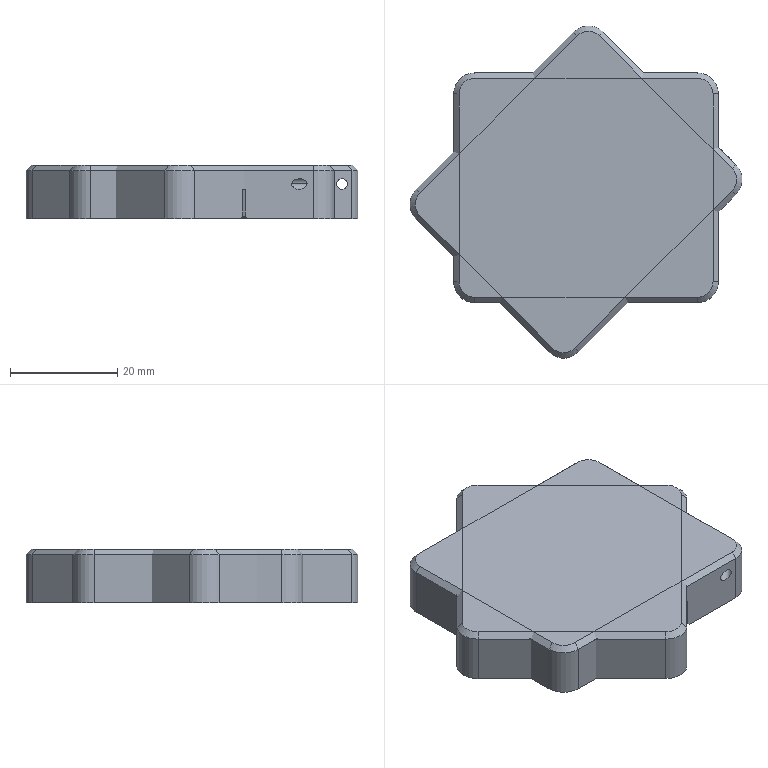NC program | NX | posted with a generic post | part box 61.954 x 61.954 x 10 mm
Lines 1286 to 2951 of 3041, first 1362 of 1662 lines:
(PLANAR_MILL_2 , TOOL : D3精光)
N2540 T03 M6
N2542 G54
N2544 G17 G0 G90 X3.83 Y-28.399 B0. C0. S3500 M3
N2546 G43 Z30. H3
N2548 Z1.
N2550 G94 G1 X3.777 Y-28.323 Z0.995 F600.
N2552 X3.672 Y-28.218 Z0.987
N2554 X3.52 Y-28.112 Z0.978
N2556 X3.349 Y-28.039 Z0.968
N2558 X3.167 Y-28.002 Z0.958
N2560 X2.981 Z0.948
N2562 X2.8 Y-28.039 Z0.939
N2564 X2.629 Y-28.112 Z0.929
N2566 X2.476 Y-28.218 Z0.919
N2568 X2.371 Y-28.323 Z0.912
N2570 X2.266 Y-28.475 Z0.902
N2572 X2.193 Y-28.646 Z0.892
N2574 X2.156 Y-28.828 Z0.882
N2576 Y-29.013 Z0.873
N2578 X2.193 Y-29.195 Z0.863
N2580 X2.266 Y-29.366 Z0.853
N2582 X2.371 Y-29.519 Z0.843
N2584 X2.476 Y-29.624 Z0.836
N2586 X2.629 Y-29.729 Z0.826
N2588 X2.8 Y-29.802 Z0.816
N2590 X2.981 Y-29.839 Z0.806
N2592 X3.167 Z0.797
N2594 X3.349 Y-29.802 Z0.787
N2596 X3.52 Y-29.729 Z0.777
N2598 X3.672 Y-29.624 Z0.768
N2600 X3.777 Y-29.519 Z0.76
N2602 X3.883 Y-29.366 Z0.75
N2604 X3.955 Y-29.195 Z0.74
N2606 X3.993 Y-29.013 Z0.731
N2608 Y-28.828 Z0.721
N2610 X3.955 Y-28.646 Z0.711
N2612 X3.883 Y-28.475 Z0.701
N2614 X3.777 Y-28.323 Z0.692
N2616 X3.672 Y-28.218 Z0.684
N2618 X3.52 Y-28.112 Z0.674
N2620 X3.349 Y-28.039 Z0.664
N2622 X3.167 Y-28.002 Z0.655
N2624 X2.981 Z0.645
N2626 X2.8 Y-28.039 Z0.635
N2628 X2.629 Y-28.112 Z0.626
N2630 X2.476 Y-28.218 Z0.616
N2632 X2.371 Y-28.323 Z0.608
N2634 X2.266 Y-28.475 Z0.598
N2636 X2.193 Y-28.646 Z0.589
N2638 X2.156 Y-28.828 Z0.579
N2640 Y-29.013 Z0.569
N2642 X2.193 Y-29.195 Z0.559
N2644 X2.266 Y-29.366 Z0.55
N2646 X2.371 Y-29.519 Z0.54
N2648 X2.476 Y-29.624 Z0.532
N2650 X2.629 Y-29.729 Z0.522
N2652 X2.8 Y-29.802 Z0.513
N2654 X2.981 Y-29.839 Z0.503
N2656 X3.167 Z0.493
N2658 X3.349 Y-29.802 Z0.484
N2660 X3.52 Y-29.729 Z0.474
N2662 X3.672 Y-29.624 Z0.464
N2664 X3.777 Y-29.519 Z0.456
N2666 X3.883 Y-29.366 Z0.447
N2668 X3.955 Y-29.195 Z0.437
N2670 X3.993 Y-29.013 Z0.427
N2672 Y-28.828 Z0.417
N2674 X3.955 Y-28.646 Z0.408
N2676 X3.883 Y-28.475 Z0.398
N2678 X3.777 Y-28.323 Z0.388
N2680 X3.672 Y-28.218 Z0.38
N2682 X3.52 Y-28.112 Z0.371
N2684 X3.349 Y-28.039 Z0.361
N2686 X3.167 Y-28.002 Z0.351
N2688 X2.981 Z0.342
N2690 X2.8 Y-28.039 Z0.332
N2692 X2.629 Y-28.112 Z0.322
N2694 X2.476 Y-28.218 Z0.312
N2696 X2.371 Y-28.323 Z0.305
N2698 X2.266 Y-28.475 Z0.295
N2700 X2.193 Y-28.646 Z0.285
N2702 X2.156 Y-28.828 Z0.275
N2704 Y-29.013 Z0.266
N2706 X2.193 Y-29.195 Z0.256
N2708 X2.266 Y-29.366 Z0.246
N2710 X2.371 Y-29.519 Z0.237
N2712 X2.476 Y-29.624 Z0.229
N2714 X2.629 Y-29.729 Z0.219
N2716 X2.8 Y-29.802 Z0.209
N2718 X2.981 Y-29.839 Z0.2
N2720 X3.167 Z0.19
N2722 X3.349 Y-29.802 Z0.18
N2724 X3.52 Y-29.729 Z0.17
N2726 X3.672 Y-29.624 Z0.161
N2728 X3.777 Y-29.519 Z0.153
N2730 X3.883 Y-29.366 Z0.143
N2732 X3.955 Y-29.195 Z0.133
N2734 X3.993 Y-29.013 Z0.124
N2736 Y-28.828 Z0.114
N2738 X3.955 Y-28.646 Z0.104
N2740 X3.883 Y-28.475 Z0.095
N2742 X3.777 Y-28.323 Z0.085
N2744 X3.672 Y-28.218 Z0.077
N2746 X3.52 Y-28.112 Z0.067
N2748 X3.349 Y-28.039 Z0.058
N2750 X3.167 Y-28.002 Z0.048
N2752 X2.981 Z0.038
N2754 X2.8 Y-28.039 Z0.028
N2756 X2.629 Y-28.112 Z0.019
N2758 X2.476 Y-28.218 Z0.009
N2760 X2.371 Y-28.323 Z0.001
N2762 X2.266 Y-28.475 Z-0.009
N2764 X2.193 Y-28.646 Z-0.018
N2766 X2.156 Y-28.828 Z-0.028
N2768 Y-29.013 Z-0.038
N2770 X2.193 Y-29.195 Z-0.047
N2772 X2.266 Y-29.366 Z-0.057
N2774 X2.371 Y-29.519 Z-0.067
N2776 X2.476 Y-29.624 Z-0.075
N2778 X2.629 Y-29.729 Z-0.084
N2780 X2.8 Y-29.802 Z-0.094
N2782 X2.981 Y-29.839 Z-0.104
N2784 X3.167 Z-0.114
N2786 X3.349 Y-29.802 Z-0.123
N2788 X3.52 Y-29.729 Z-0.133
N2790 X3.672 Y-29.624 Z-0.143
N2792 X3.777 Y-29.519 Z-0.151
N2794 X3.883 Y-29.366 Z-0.16
N2796 X3.955 Y-29.195 Z-0.17
N2798 X3.993 Y-29.013 Z-0.18
N2800 Y-28.828 Z-0.189
N2802 X3.955 Y-28.646 Z-0.199
N2804 X3.883 Y-28.475 Z-0.209
N2806 X3.777 Y-28.323 Z-0.219
N2808 X3.672 Y-28.218 Z-0.226
N2810 X3.52 Y-28.112 Z-0.236
N2812 X3.349 Y-28.039 Z-0.246
N2814 X3.167 Y-28.002 Z-0.256
N2816 X2.981 Z-0.265
N2818 X2.8 Y-28.039 Z-0.275
N2820 X2.629 Y-28.112 Z-0.285
N2822 X2.476 Y-28.218 Z-0.294
N2824 X2.371 Y-28.323 Z-0.302
N2826 X2.266 Y-28.475 Z-0.312
N2828 X2.193 Y-28.646 Z-0.322
N2830 X2.156 Y-28.828 Z-0.331
N2832 Y-29.013 Z-0.341
N2834 X2.193 Y-29.195 Z-0.351
N2836 X2.266 Y-29.366 Z-0.361
N2838 X2.371 Y-29.519 Z-0.37
N2840 X2.476 Y-29.624 Z-0.378
N2842 X2.629 Y-29.729 Z-0.388
N2844 X2.8 Y-29.802 Z-0.398
N2846 X2.981 Y-29.839 Z-0.407
N2848 X3.167 Z-0.417
N2850 X3.349 Y-29.802 Z-0.427
N2852 X3.52 Y-29.729 Z-0.436
N2854 X3.672 Y-29.624 Z-0.446
N2856 X3.777 Y-29.519 Z-0.454
N2858 X3.883 Y-29.366 Z-0.464
N2860 X3.955 Y-29.195 Z-0.473
N2862 X3.993 Y-29.013 Z-0.483
N2864 Y-28.828 Z-0.493
N2866 X3.955 Y-28.646 Z-0.503
N2868 X3.883 Y-28.475 Z-0.512
N2870 X3.777 Y-28.323 Z-0.522
N2872 X3.672 Y-28.218 Z-0.53
N2874 X3.52 Y-28.112 Z-0.54
N2876 X3.349 Y-28.039 Z-0.549
N2878 X3.167 Y-28.002 Z-0.559
N2880 X2.981 Z-0.569
N2882 X2.8 Y-28.039 Z-0.578
N2884 X2.629 Y-28.112 Z-0.588
N2886 X2.476 Y-28.218 Z-0.598
N2888 X2.371 Y-28.323 Z-0.606
N2890 X2.266 Y-28.475 Z-0.615
N2892 X2.193 Y-28.646 Z-0.625
N2894 X2.156 Y-28.828 Z-0.635
N2896 Y-29.013 Z-0.645
N2898 X2.193 Y-29.195 Z-0.654
N2900 X2.266 Y-29.366 Z-0.664
N2902 X2.371 Y-29.519 Z-0.674
N2904 X2.476 Y-29.624 Z-0.682
N2906 X2.629 Y-29.729 Z-0.691
N2908 X2.8 Y-29.802 Z-0.701
N2910 X2.981 Y-29.839 Z-0.711
N2912 X3.167 Z-0.72
N2914 X3.349 Y-29.802 Z-0.73
N2916 X3.52 Y-29.729 Z-0.74
N2918 X3.672 Y-29.624 Z-0.75
N2920 X3.777 Y-29.519 Z-0.757
N2922 X3.883 Y-29.366 Z-0.767
N2924 X3.955 Y-29.195 Z-0.777
N2926 X3.993 Y-29.013 Z-0.787
N2928 Y-28.828 Z-0.796
N2930 X3.955 Y-28.646 Z-0.806
N2932 X3.883 Y-28.475 Z-0.816
N2934 X3.777 Y-28.323 Z-0.825
N2936 X3.672 Y-28.218 Z-0.833
N2938 X3.52 Y-28.112 Z-0.843
N2940 X3.349 Y-28.039 Z-0.853
N2942 X3.167 Y-28.002 Z-0.862
N2944 X2.981 Z-0.872
N2946 X2.8 Y-28.039 Z-0.882
N2948 X2.629 Y-28.112 Z-0.892
N2950 X2.476 Y-28.218 Z-0.901
N2952 X2.371 Y-28.323 Z-0.909
N2954 X2.266 Y-28.475 Z-0.919
N2956 X2.193 Y-28.646 Z-0.929
N2958 X2.156 Y-28.828 Z-0.938
N2960 Y-29.013 Z-0.948
N2962 X2.193 Y-29.195 Z-0.958
N2964 X2.266 Y-29.366 Z-0.967
N2966 X2.371 Y-29.519 Z-0.977
N2968 X2.476 Y-29.624 Z-0.985
N2970 X2.629 Y-29.729 Z-0.995
N2972 X2.8 Y-29.802 Z-1.004
N2974 X2.981 Y-29.839 Z-1.014
N2976 X3.167 Z-1.024
N2978 X3.349 Y-29.802 Z-1.034
N2980 X3.52 Y-29.729 Z-1.043
N2982 X3.672 Y-29.624 Z-1.053
N2984 X3.777 Y-29.519 Z-1.061
N2986 X3.883 Y-29.366 Z-1.071
N2988 X3.955 Y-29.195 Z-1.08
N2990 X3.993 Y-29.013 Z-1.09
N2992 Y-28.828 Z-1.1
N2994 X3.955 Y-28.646 Z-1.109
N2996 X3.883 Y-28.475 Z-1.119
N2998 X3.777 Y-28.323 Z-1.129
N3000 X3.672 Y-28.218 Z-1.137
N3002 X3.52 Y-28.112 Z-1.146
N3004 X3.349 Y-28.039 Z-1.156
N3006 X3.167 Y-28.002 Z-1.166
N3008 X2.981 Z-1.176
N3010 X2.8 Y-28.039 Z-1.185
N3012 X2.629 Y-28.112 Z-1.195
N3014 X2.476 Y-28.218 Z-1.205
N3016 X2.371 Y-28.323 Z-1.213
N3018 X2.266 Y-28.475 Z-1.222
N3020 X2.193 Y-28.646 Z-1.232
N3022 X2.156 Y-28.828 Z-1.242
N3024 Y-29.013 Z-1.251
N3026 X2.193 Y-29.195 Z-1.261
N3028 X2.266 Y-29.366 Z-1.271
N3030 X2.371 Y-29.519 Z-1.281
N3032 X2.476 Y-29.624 Z-1.288
N3034 X2.629 Y-29.729 Z-1.298
N3036 X2.8 Y-29.802 Z-1.308
N3038 X2.981 Y-29.839 Z-1.318
N3040 X3.167 Z-1.327
N3042 X3.349 Y-29.802 Z-1.337
N3044 X3.52 Y-29.729 Z-1.347
N3046 X3.672 Y-29.624 Z-1.356
N3048 X3.777 Y-29.519 Z-1.364
N3050 X3.883 Y-29.366 Z-1.374
N3052 X3.955 Y-29.195 Z-1.384
N3054 X3.993 Y-29.013 Z-1.393
N3056 Y-28.828 Z-1.403
N3058 X3.955 Y-28.646 Z-1.413
N3060 X3.883 Y-28.475 Z-1.423
N3062 X3.777 Y-28.323 Z-1.432
N3064 X3.672 Y-28.218 Z-1.44
N3066 X3.52 Y-28.112 Z-1.45
N3068 X3.349 Y-28.039 Z-1.46
N3070 X3.167 Y-28.002 Z-1.469
N3072 X2.981 Z-1.479
N3074 X2.8 Y-28.039 Z-1.489
N3076 X2.629 Y-28.112 Z-1.498
N3078 X2.476 Y-28.218 Z-1.508
N3080 X2.371 Y-28.323 Z-1.516
N3082 X2.266 Y-28.475 Z-1.526
N3084 X2.193 Y-28.646 Z-1.535
N3086 X2.156 Y-28.828 Z-1.545
N3088 Y-29.013 Z-1.555
N3090 X2.193 Y-29.195 Z-1.565
N3092 X2.266 Y-29.366 Z-1.574
N3094 X2.371 Y-29.519 Z-1.584
N3096 X2.476 Y-29.624 Z-1.592
N3098 X2.629 Y-29.729 Z-1.602
N3100 X2.8 Y-29.802 Z-1.611
N3102 X2.981 Y-29.839 Z-1.621
N3104 X3.167 Z-1.631
N3106 X3.349 Y-29.802 Z-1.64
N3108 X3.52 Y-29.729 Z-1.65
N3110 X3.672 Y-29.624 Z-1.66
N3112 X3.777 Y-29.519 Z-1.668
N3114 X3.883 Y-29.366 Z-1.677
N3116 X3.955 Y-29.195 Z-1.687
N3118 X3.993 Y-29.013 Z-1.697
N3120 Y-28.828 Z-1.707
N3122 X3.955 Y-28.646 Z-1.716
N3124 X3.883 Y-28.475 Z-1.726
N3126 X3.777 Y-28.323 Z-1.736
N3128 X3.672 Y-28.218 Z-1.744
N3130 X3.52 Y-28.112 Z-1.753
N3132 X3.349 Y-28.039 Z-1.763
N3134 X3.167 Y-28.002 Z-1.773
N3136 X2.981 Z-1.782
N3138 X2.8 Y-28.039 Z-1.792
N3140 X2.629 Y-28.112 Z-1.802
N3142 X2.476 Y-28.218 Z-1.812
N3144 X2.371 Y-28.323 Z-1.819
N3146 X2.266 Y-28.475 Z-1.829
N3148 X2.193 Y-28.646 Z-1.839
N3150 X2.156 Y-28.828 Z-1.849
N3152 Y-29.013 Z-1.858
N3154 X2.193 Y-29.195 Z-1.868
N3156 X2.266 Y-29.366 Z-1.878
N3158 X2.371 Y-29.519 Z-1.888
N3160 X2.476 Y-29.624 Z-1.895
N3162 X2.629 Y-29.729 Z-1.905
N3164 X2.8 Y-29.802 Z-1.915
N3166 X2.981 Y-29.839 Z-1.924
N3168 X3.167 Z-1.934
N3170 X3.349 Y-29.802 Z-1.944
N3172 X3.52 Y-29.729 Z-1.954
N3174 X3.672 Y-29.624 Z-1.963
N3176 X3.777 Y-29.519 Z-1.971
N3178 X3.883 Y-29.366 Z-1.981
N3180 X3.955 Y-29.195 Z-1.991
N3182 X3.993 Y-29.013 Z-2.
N3184 Y-28.828 Z-2.01
N3186 X3.955 Y-28.646 Z-2.02
N3188 X3.883 Y-28.475 Z-2.03
N3190 X3.777 Y-28.323 Z-2.039
N3192 X3.672 Y-28.218 Z-2.047
N3194 X3.52 Y-28.112 Z-2.057
N3196 X3.349 Y-28.039 Z-2.066
N3198 X3.167 Y-28.002 Z-2.076
N3200 X2.981 Z-2.086
N3202 X2.8 Y-28.039 Z-2.096
N3204 X2.629 Y-28.112 Z-2.105
N3206 X2.476 Y-28.218 Z-2.115
N3208 X2.371 Y-28.323 Z-2.123
N3210 X2.266 Y-28.475 Z-2.133
N3212 X2.193 Y-28.646 Z-2.142
N3214 X2.156 Y-28.828 Z-2.152
N3216 Y-29.013 Z-2.162
N3218 X2.193 Y-29.195 Z-2.171
N3220 X2.266 Y-29.366 Z-2.181
N3222 X2.371 Y-29.519 Z-2.191
N3224 X2.476 Y-29.624 Z-2.199
N3226 X2.629 Y-29.729 Z-2.208
N3228 X2.8 Y-29.802 Z-2.218
N3230 X2.981 Y-29.839 Z-2.228
N3232 X3.167 Z-2.238
N3234 X3.349 Y-29.802 Z-2.247
N3236 X3.52 Y-29.729 Z-2.257
N3238 X3.672 Y-29.624 Z-2.267
N3240 X3.777 Y-29.519 Z-2.275
N3242 X3.883 Y-29.366 Z-2.284
N3244 X3.955 Y-29.195 Z-2.294
N3246 X3.993 Y-29.013 Z-2.304
N3248 Y-28.828 Z-2.313
N3250 X3.955 Y-28.646 Z-2.323
N3252 X3.883 Y-28.475 Z-2.333
N3254 X3.777 Y-28.323 Z-2.343
N3256 X3.672 Y-28.218 Z-2.35
N3258 X3.52 Y-28.112 Z-2.36
N3260 X3.349 Y-28.039 Z-2.37
N3262 X3.167 Y-28.002 Z-2.38
N3264 X2.981 Z-2.389
N3266 X2.8 Y-28.039 Z-2.399
N3268 X2.629 Y-28.112 Z-2.409
N3270 X2.476 Y-28.218 Z-2.419
N3272 X2.371 Y-28.323 Z-2.426
N3274 X2.266 Y-28.475 Z-2.436
N3276 X2.193 Y-28.646 Z-2.446
N3278 X2.156 Y-28.828 Z-2.455
N3280 Y-29.013 Z-2.465
N3282 X2.193 Y-29.195 Z-2.475
N3284 X2.266 Y-29.366 Z-2.485
N3286 X2.371 Y-29.519 Z-2.494
N3288 X2.476 Y-29.624 Z-2.502
N3290 X2.629 Y-29.729 Z-2.512
N3292 X2.8 Y-29.802 Z-2.522
N3294 X2.981 Y-29.839 Z-2.531
N3296 X3.167 Z-2.541
N3298 X3.349 Y-29.802 Z-2.551
N3300 X3.52 Y-29.729 Z-2.561
N3302 X3.672 Y-29.624 Z-2.57
N3304 X3.777 Y-29.519 Z-2.578
N3306 X3.883 Y-29.366 Z-2.588
N3308 X3.955 Y-29.195 Z-2.597
N3310 X3.993 Y-29.013 Z-2.607
N3312 Y-28.828 Z-2.617
N3314 X3.955 Y-28.646 Z-2.627
N3316 X3.883 Y-28.475 Z-2.636
N3318 X3.777 Y-28.323 Z-2.646
N3320 X3.725 Y-28.27 Z-2.65
N3322 G3 X2.424 Y-28.27 R0.92
N3324 X3.725 Y-28.27 R-0.92
N3326 G1 Z-1.65
N3328 G0 Z30.
N3330 X27.067 Y-4.694
N3332 Z1.
N3334 G1 X27.12 Y-4.77 Z0.995
N3336 X27.225 Y-4.875 Z0.987
N3338 X27.378 Y-4.98 Z0.978
N3340 X27.548 Y-5.053 Z0.968
N3342 X27.73 Y-5.09 Z0.958
N3344 X27.916 Z0.948
N3346 X28.098 Y-5.053 Z0.939
N3348 X28.268 Y-4.98 Z0.929
N3350 X28.421 Y-4.875 Z0.919
N3352 X28.526 Y-4.77 Z0.912
N3354 X28.632 Y-4.617 Z0.902
N3356 X28.704 Y-4.446 Z0.892
N3358 X28.741 Y-4.265 Z0.882
N3360 Y-4.079 Z0.873
N3362 X28.704 Y-3.897 Z0.863
N3364 X28.632 Y-3.727 Z0.853
N3366 X28.526 Y-3.574 Z0.843
N3368 X28.421 Y-3.469 Z0.836
N3370 X28.268 Y-3.363 Z0.826
N3372 X28.098 Y-3.291 Z0.816
N3374 X27.916 Y-3.254 Z0.806
N3376 X27.73 Z0.797
N3378 X27.548 Y-3.291 Z0.787
N3380 X27.378 Y-3.363 Z0.777
N3382 X27.225 Y-3.469 Z0.768
N3384 X27.12 Y-3.574 Z0.76
N3386 X27.014 Y-3.727 Z0.75
N3388 X26.942 Y-3.897 Z0.74
N3390 X26.905 Y-4.079 Z0.731
N3392 Y-4.265 Z0.721
N3394 X26.942 Y-4.446 Z0.711
N3396 X27.014 Y-4.617 Z0.701
N3398 X27.12 Y-4.77 Z0.692
N3400 X27.225 Y-4.875 Z0.684
N3402 X27.378 Y-4.98 Z0.674
N3404 X27.548 Y-5.053 Z0.664
N3406 X27.73 Y-5.09 Z0.655
N3408 X27.916 Z0.645
N3410 X28.098 Y-5.053 Z0.635
N3412 X28.268 Y-4.98 Z0.626
N3414 X28.421 Y-4.875 Z0.616
N3416 X28.526 Y-4.77 Z0.608
N3418 X28.632 Y-4.617 Z0.598
N3420 X28.704 Y-4.446 Z0.589
N3422 X28.741 Y-4.265 Z0.579
N3424 Y-4.079 Z0.569
N3426 X28.704 Y-3.897 Z0.559
N3428 X28.632 Y-3.727 Z0.55
N3430 X28.526 Y-3.574 Z0.54
N3432 X28.421 Y-3.469 Z0.532
N3434 X28.268 Y-3.363 Z0.522
N3436 X28.098 Y-3.291 Z0.513
N3438 X27.916 Y-3.254 Z0.503
N3440 X27.73 Z0.493
N3442 X27.548 Y-3.291 Z0.484
N3444 X27.378 Y-3.363 Z0.474
N3446 X27.225 Y-3.469 Z0.464
N3448 X27.12 Y-3.574 Z0.456
N3450 X27.014 Y-3.727 Z0.447
N3452 X26.942 Y-3.897 Z0.437
N3454 X26.905 Y-4.079 Z0.427
N3456 Y-4.265 Z0.417
N3458 X26.942 Y-4.446 Z0.408
N3460 X27.014 Y-4.617 Z0.398
N3462 X27.12 Y-4.77 Z0.388
N3464 X27.225 Y-4.875 Z0.38
N3466 X27.378 Y-4.98 Z0.371
N3468 X27.548 Y-5.053 Z0.361
N3470 X27.73 Y-5.09 Z0.351
N3472 X27.916 Z0.342
N3474 X28.098 Y-5.053 Z0.332
N3476 X28.268 Y-4.98 Z0.322
N3478 X28.421 Y-4.875 Z0.312
N3480 X28.526 Y-4.77 Z0.305
N3482 X28.632 Y-4.617 Z0.295
N3484 X28.704 Y-4.446 Z0.285
N3486 X28.741 Y-4.265 Z0.275
N3488 Y-4.079 Z0.266
N3490 X28.704 Y-3.897 Z0.256
N3492 X28.632 Y-3.727 Z0.246
N3494 X28.526 Y-3.574 Z0.237
N3496 X28.421 Y-3.469 Z0.229
N3498 X28.268 Y-3.363 Z0.219
N3500 X28.098 Y-3.291 Z0.209
N3502 X27.916 Y-3.254 Z0.2
N3504 X27.73 Z0.19
N3506 X27.548 Y-3.291 Z0.18
N3508 X27.378 Y-3.363 Z0.17
N3510 X27.225 Y-3.469 Z0.161
N3512 X27.12 Y-3.574 Z0.153
N3514 X27.014 Y-3.727 Z0.143
N3516 X26.942 Y-3.897 Z0.133
N3518 X26.905 Y-4.079 Z0.124
N3520 Y-4.265 Z0.114
N3522 X26.942 Y-4.446 Z0.104
N3524 X27.014 Y-4.617 Z0.095
N3526 X27.12 Y-4.77 Z0.085
N3528 X27.225 Y-4.875 Z0.077
N3530 X27.378 Y-4.98 Z0.067
N3532 X27.548 Y-5.053 Z0.058
N3534 X27.73 Y-5.09 Z0.048
N3536 X27.916 Z0.038
N3538 X28.098 Y-5.053 Z0.028
N3540 X28.268 Y-4.98 Z0.019
N3542 X28.421 Y-4.875 Z0.009
N3544 X28.526 Y-4.77 Z0.001
N3546 X28.632 Y-4.617 Z-0.009
N3548 X28.704 Y-4.446 Z-0.018
N3550 X28.741 Y-4.265 Z-0.028
N3552 Y-4.079 Z-0.038
N3554 X28.704 Y-3.897 Z-0.047
N3556 X28.632 Y-3.727 Z-0.057
N3558 X28.526 Y-3.574 Z-0.067
N3560 X28.421 Y-3.469 Z-0.075
N3562 X28.268 Y-3.363 Z-0.084
N3564 X28.098 Y-3.291 Z-0.094
N3566 X27.916 Y-3.254 Z-0.104
N3568 X27.73 Z-0.114
N3570 X27.548 Y-3.291 Z-0.123
N3572 X27.378 Y-3.363 Z-0.133
N3574 X27.225 Y-3.469 Z-0.143
N3576 X27.12 Y-3.574 Z-0.151
N3578 X27.014 Y-3.727 Z-0.16
N3580 X26.942 Y-3.897 Z-0.17
N3582 X26.905 Y-4.079 Z-0.18
N3584 Y-4.265 Z-0.189
N3586 X26.942 Y-4.446 Z-0.199
N3588 X27.014 Y-4.617 Z-0.209
N3590 X27.12 Y-4.77 Z-0.219
N3592 X27.225 Y-4.875 Z-0.226
N3594 X27.378 Y-4.98 Z-0.236
N3596 X27.548 Y-5.053 Z-0.246
N3598 X27.73 Y-5.09 Z-0.256
N3600 X27.916 Z-0.265
N3602 X28.098 Y-5.053 Z-0.275
N3604 X28.268 Y-4.98 Z-0.285
N3606 X28.421 Y-4.875 Z-0.294
N3608 X28.526 Y-4.77 Z-0.302
N3610 X28.632 Y-4.617 Z-0.312
N3612 X28.704 Y-4.446 Z-0.322
N3614 X28.741 Y-4.265 Z-0.331
N3616 Y-4.079 Z-0.341
N3618 X28.704 Y-3.897 Z-0.351
N3620 X28.632 Y-3.727 Z-0.361
N3622 X28.526 Y-3.574 Z-0.37
N3624 X28.421 Y-3.469 Z-0.378
N3626 X28.268 Y-3.363 Z-0.388
N3628 X28.098 Y-3.291 Z-0.398
N3630 X27.916 Y-3.254 Z-0.407
N3632 X27.73 Z-0.417
N3634 X27.548 Y-3.291 Z-0.427
N3636 X27.378 Y-3.363 Z-0.436
N3638 X27.225 Y-3.469 Z-0.446
N3640 X27.12 Y-3.574 Z-0.454
N3642 X27.014 Y-3.727 Z-0.464
N3644 X26.942 Y-3.897 Z-0.473
N3646 X26.905 Y-4.079 Z-0.483
N3648 Y-4.265 Z-0.493
N3650 X26.942 Y-4.446 Z-0.503
N3652 X27.014 Y-4.617 Z-0.512
N3654 X27.12 Y-4.77 Z-0.522
N3656 X27.225 Y-4.875 Z-0.53
N3658 X27.378 Y-4.98 Z-0.54
N3660 X27.548 Y-5.053 Z-0.549
N3662 X27.73 Y-5.09 Z-0.559
N3664 X27.916 Z-0.569
N3666 X28.098 Y-5.053 Z-0.578
N3668 X28.268 Y-4.98 Z-0.588
N3670 X28.421 Y-4.875 Z-0.598
N3672 X28.526 Y-4.77 Z-0.606
N3674 X28.632 Y-4.617 Z-0.615
N3676 X28.704 Y-4.446 Z-0.625
N3678 X28.741 Y-4.265 Z-0.635
N3680 Y-4.079 Z-0.645
N3682 X28.704 Y-3.897 Z-0.654
N3684 X28.632 Y-3.727 Z-0.664
N3686 X28.526 Y-3.574 Z-0.674
N3688 X28.421 Y-3.469 Z-0.682
N3690 X28.268 Y-3.363 Z-0.691
N3692 X28.098 Y-3.291 Z-0.701
N3694 X27.916 Y-3.254 Z-0.711
N3696 X27.73 Z-0.72
N3698 X27.548 Y-3.291 Z-0.73
N3700 X27.378 Y-3.363 Z-0.74
N3702 X27.225 Y-3.469 Z-0.75
N3704 X27.12 Y-3.574 Z-0.757
N3706 X27.014 Y-3.727 Z-0.767
N3708 X26.942 Y-3.897 Z-0.777
N3710 X26.905 Y-4.079 Z-0.787
N3712 Y-4.265 Z-0.796
N3714 X26.942 Y-4.446 Z-0.806
N3716 X27.014 Y-4.617 Z-0.816
N3718 X27.12 Y-4.77 Z-0.825
N3720 X27.225 Y-4.875 Z-0.833
N3722 X27.378 Y-4.98 Z-0.843
N3724 X27.548 Y-5.053 Z-0.853
N3726 X27.73 Y-5.09 Z-0.862
N3728 X27.916 Z-0.872
N3730 X28.098 Y-5.053 Z-0.882
N3732 X28.268 Y-4.98 Z-0.892
N3734 X28.421 Y-4.875 Z-0.901
N3736 X28.526 Y-4.77 Z-0.909
N3738 X28.632 Y-4.617 Z-0.919
N3740 X28.704 Y-4.446 Z-0.929
N3742 X28.741 Y-4.265 Z-0.938
N3744 Y-4.079 Z-0.948
N3746 X28.704 Y-3.897 Z-0.958
N3748 X28.632 Y-3.727 Z-0.967
N3750 X28.526 Y-3.574 Z-0.977
N3752 X28.421 Y-3.469 Z-0.985
N3754 X28.268 Y-3.363 Z-0.995
N3756 X28.098 Y-3.291 Z-1.004
N3758 X27.916 Y-3.254 Z-1.014
N3760 X27.73 Z-1.024
N3762 X27.548 Y-3.291 Z-1.034
N3764 X27.378 Y-3.363 Z-1.043
N3766 X27.225 Y-3.469 Z-1.053
N3768 X27.12 Y-3.574 Z-1.061
N3770 X27.014 Y-3.727 Z-1.071
N3772 X26.942 Y-3.897 Z-1.08
N3774 X26.905 Y-4.079 Z-1.09
N3776 Y-4.265 Z-1.1
N3778 X26.942 Y-4.446 Z-1.109
N3780 X27.014 Y-4.617 Z-1.119
N3782 X27.12 Y-4.77 Z-1.129
N3784 X27.225 Y-4.875 Z-1.137
N3786 X27.378 Y-4.98 Z-1.146
N3788 X27.548 Y-5.053 Z-1.156
N3790 X27.73 Y-5.09 Z-1.166
N3792 X27.916 Z-1.176
N3794 X28.098 Y-5.053 Z-1.185
N3796 X28.268 Y-4.98 Z-1.195
N3798 X28.421 Y-4.875 Z-1.205
N3800 X28.526 Y-4.77 Z-1.213
N3802 X28.632 Y-4.617 Z-1.222
N3804 X28.704 Y-4.446 Z-1.232
N3806 X28.741 Y-4.265 Z-1.242
N3808 Y-4.079 Z-1.251
N3810 X28.704 Y-3.897 Z-1.261
N3812 X28.632 Y-3.727 Z-1.271
N3814 X28.526 Y-3.574 Z-1.281
N3816 X28.421 Y-3.469 Z-1.288
N3818 X28.268 Y-3.363 Z-1.298
N3820 X28.098 Y-3.291 Z-1.308
N3822 X27.916 Y-3.254 Z-1.318
N3824 X27.73 Z-1.327
N3826 X27.548 Y-3.291 Z-1.337
N3828 X27.378 Y-3.363 Z-1.347
N3830 X27.225 Y-3.469 Z-1.356
N3832 X27.12 Y-3.574 Z-1.364
N3834 X27.014 Y-3.727 Z-1.374
N3836 X26.942 Y-3.897 Z-1.384
N3838 X26.905 Y-4.079 Z-1.393
N3840 Y-4.265 Z-1.403
N3842 X26.942 Y-4.446 Z-1.413
N3844 X27.014 Y-4.617 Z-1.423
N3846 X27.12 Y-4.77 Z-1.432
N3848 X27.225 Y-4.875 Z-1.44
N3850 X27.378 Y-4.98 Z-1.45
N3852 X27.548 Y-5.053 Z-1.46
N3854 X27.73 Y-5.09 Z-1.469
N3856 X27.916 Z-1.479
N3858 X28.098 Y-5.053 Z-1.489
N3860 X28.268 Y-4.98 Z-1.498
N3862 X28.421 Y-4.875 Z-1.508
N3864 X28.526 Y-4.77 Z-1.516
N3866 X28.632 Y-4.617 Z-1.526
N3868 X28.704 Y-4.446 Z-1.535
N3870 X28.741 Y-4.265 Z-1.545
N3872 Y-4.079 Z-1.555
N3874 X28.704 Y-3.897 Z-1.565
N3876 X28.632 Y-3.727 Z-1.574
N3878 X28.526 Y-3.574 Z-1.584
N3880 X28.421 Y-3.469 Z-1.592
N3882 X28.268 Y-3.363 Z-1.602
N3884 X28.098 Y-3.291 Z-1.611
N3886 X27.916 Y-3.254 Z-1.621
N3888 X27.73 Z-1.631
N3890 X27.548 Y-3.291 Z-1.64
N3892 X27.378 Y-3.363 Z-1.65
N3894 X27.225 Y-3.469 Z-1.66
N3896 X27.12 Y-3.574 Z-1.668
N3898 X27.014 Y-3.727 Z-1.677
N3900 X26.942 Y-3.897 Z-1.687
N3902 X26.905 Y-4.079 Z-1.697
N3904 Y-4.265 Z-1.707
N3906 X26.942 Y-4.446 Z-1.716
N3908 X27.014 Y-4.617 Z-1.726
N3910 X27.12 Y-4.77 Z-1.736
N3912 X27.225 Y-4.875 Z-1.744
N3914 X27.378 Y-4.98 Z-1.753
N3916 X27.548 Y-5.053 Z-1.763
N3918 X27.73 Y-5.09 Z-1.773
N3920 X27.916 Z-1.782
N3922 X28.098 Y-5.053 Z-1.792
N3924 X28.268 Y-4.98 Z-1.802
N3926 X28.421 Y-4.875 Z-1.812
N3928 X28.526 Y-4.77 Z-1.819
N3930 X28.632 Y-4.617 Z-1.829
N3932 X28.704 Y-4.446 Z-1.839
N3934 X28.741 Y-4.265 Z-1.849
N3936 Y-4.079 Z-1.858
N3938 X28.704 Y-3.897 Z-1.868
N3940 X28.632 Y-3.727 Z-1.878
N3942 X28.526 Y-3.574 Z-1.888
N3944 X28.421 Y-3.469 Z-1.895
N3946 X28.268 Y-3.363 Z-1.905
N3948 X28.098 Y-3.291 Z-1.915
N3950 X27.916 Y-3.254 Z-1.924
N3952 X27.73 Z-1.934
N3954 X27.548 Y-3.291 Z-1.944
N3956 X27.378 Y-3.363 Z-1.954
N3958 X27.225 Y-3.469 Z-1.963
N3960 X27.12 Y-3.574 Z-1.971
N3962 X27.014 Y-3.727 Z-1.981
N3964 X26.942 Y-3.897 Z-1.991
N3966 X26.905 Y-4.079 Z-2.
N3968 Y-4.265 Z-2.01
N3970 X26.942 Y-4.446 Z-2.02
N3972 X27.014 Y-4.617 Z-2.03
N3974 X27.12 Y-4.77 Z-2.039
N3976 X27.225 Y-4.875 Z-2.047
N3978 X27.378 Y-4.98 Z-2.057
N3980 X27.548 Y-5.053 Z-2.066
N3982 X27.73 Y-5.09 Z-2.076
N3984 X27.916 Z-2.086
N3986 X28.098 Y-5.053 Z-2.096
N3988 X28.268 Y-4.98 Z-2.105
N3990 X28.421 Y-4.875 Z-2.115
N3992 X28.526 Y-4.77 Z-2.123
N3994 X28.632 Y-4.617 Z-2.133
N3996 X28.704 Y-4.446 Z-2.142
N3998 X28.741 Y-4.265 Z-2.152
N4000 Y-4.079 Z-2.162
N4002 X28.704 Y-3.897 Z-2.171
N4004 X28.632 Y-3.727 Z-2.181
N4006 X28.526 Y-3.574 Z-2.191
N4008 X28.421 Y-3.469 Z-2.199
N4010 X28.268 Y-3.363 Z-2.208
N4012 X28.098 Y-3.291 Z-2.218
N4014 X27.916 Y-3.254 Z-2.228
N4016 X27.73 Z-2.238
N4018 X27.548 Y-3.291 Z-2.247
N4020 X27.378 Y-3.363 Z-2.257
N4022 X27.225 Y-3.469 Z-2.267
N4024 X27.12 Y-3.574 Z-2.275
N4026 X27.014 Y-3.727 Z-2.284
N4028 X26.942 Y-3.897 Z-2.294
N4030 X26.905 Y-4.079 Z-2.304
N4032 Y-4.265 Z-2.313
N4034 X26.942 Y-4.446 Z-2.323
N4036 X27.014 Y-4.617 Z-2.333
N4038 X27.12 Y-4.77 Z-2.343
N4040 X27.225 Y-4.875 Z-2.35
N4042 X27.378 Y-4.98 Z-2.36
N4044 X27.548 Y-5.053 Z-2.37
N4046 X27.73 Y-5.09 Z-2.38
N4048 X27.916 Z-2.389
N4050 X28.098 Y-5.053 Z-2.399
N4052 X28.268 Y-4.98 Z-2.409
N4054 X28.421 Y-4.875 Z-2.419
N4056 X28.526 Y-4.77 Z-2.426
N4058 X28.632 Y-4.617 Z-2.436
N4060 X28.704 Y-4.446 Z-2.446
N4062 X28.741 Y-4.265 Z-2.455
N4064 Y-4.079 Z-2.465
N4066 X28.704 Y-3.897 Z-2.475
N4068 X28.632 Y-3.727 Z-2.485
N4070 X28.526 Y-3.574 Z-2.494
N4072 X28.421 Y-3.469 Z-2.502
N4074 X28.268 Y-3.363 Z-2.512
N4076 X28.098 Y-3.291 Z-2.522
N4078 X27.916 Y-3.254 Z-2.531
N4080 X27.73 Z-2.541
N4082 X27.548 Y-3.291 Z-2.551
N4084 X27.378 Y-3.363 Z-2.561
N4086 X27.225 Y-3.469 Z-2.57
N4088 X27.12 Y-3.574 Z-2.578
N4090 X27.014 Y-3.727 Z-2.588
N4092 X26.942 Y-3.897 Z-2.597
N4094 X26.905 Y-4.079 Z-2.607
N4096 Y-4.265 Z-2.617
N4098 X26.942 Y-4.446 Z-2.627
N4100 X27.014 Y-4.617 Z-2.636
N4102 X27.12 Y-4.77 Z-2.646
N4104 X27.172 Y-4.822 Z-2.65
N4106 G3 X28.474 Y-4.822 R0.92
N4108 X27.172 Y-4.822 R-0.92
N4110 G1 Z-1.65
N4112 G0 Z30.
N4114 X-0.766 Y25.695
N4116 Z1.
N4118 G1 X-0.819 Y25.771 Z0.995
N4120 X-0.924 Y25.876 Z0.987
N4122 X-1.077 Y25.982 Z0.978
N4124 X-1.247 Y26.054 Z0.968
N4126 X-1.429 Y26.091 Z0.958
N4128 X-1.615 Z0.948
N4130 X-1.796 Y26.054 Z0.939
N4132 X-1.967 Y25.982 Z0.929
N4134 X-2.12 Y25.876 Z0.919
N4136 X-2.225 Y25.771 Z0.912
N4138 X-2.33 Y25.618 Z0.902
N4140 X-2.403 Y25.448 Z0.892
N4142 X-2.44 Y25.266 Z0.882
N4144 Y25.08 Z0.873
N4146 X-2.403 Y24.898 Z0.863
N4148 X-2.33 Y24.728 Z0.853
N4150 X-2.225 Y24.575 Z0.843
N4152 X-2.12 Y24.47 Z0.836
N4154 X-1.967 Y24.364 Z0.826
N4156 X-1.796 Y24.292 Z0.816
N4158 X-1.615 Y24.255 Z0.806
N4160 X-1.429 Z0.797
N4162 X-1.247 Y24.292 Z0.787
N4164 X-1.077 Y24.364 Z0.777
N4166 X-0.924 Y24.47 Z0.768
N4168 X-0.819 Y24.575 Z0.76
N4170 X-0.713 Y24.728 Z0.75
N4172 X-0.641 Y24.898 Z0.74
N4174 X-0.604 Y25.08 Z0.731
N4176 Y25.266 Z0.721
N4178 X-0.641 Y25.448 Z0.711
N4180 X-0.713 Y25.618 Z0.701
N4182 X-0.819 Y25.771 Z0.692
N4184 X-0.924 Y25.876 Z0.684
N4186 X-1.077 Y25.982 Z0.674
N4188 X-1.247 Y26.054 Z0.664
N4190 X-1.429 Y26.091 Z0.655
N4192 X-1.615 Z0.645
N4194 X-1.796 Y26.054 Z0.635
N4196 X-1.967 Y25.982 Z0.626
N4198 X-2.12 Y25.876 Z0.616
N4200 X-2.225 Y25.771 Z0.608
N4202 X-2.33 Y25.618 Z0.598
N4204 X-2.403 Y25.448 Z0.589
N4206 X-2.44 Y25.266 Z0.579
N4208 Y25.08 Z0.569
N4210 X-2.403 Y24.898 Z0.559
N4212 X-2.33 Y24.728 Z0.55
N4214 X-2.225 Y24.575 Z0.54
N4216 X-2.12 Y24.47 Z0.532
N4218 X-1.967 Y24.364 Z0.522
N4220 X-1.796 Y24.292 Z0.513
N4222 X-1.615 Y24.255 Z0.503
N4224 X-1.429 Z0.493
N4226 X-1.247 Y24.292 Z0.484
N4228 X-1.077 Y24.364 Z0.474
N4230 X-0.924 Y24.47 Z0.464
N4232 X-0.819 Y24.575 Z0.456
N4234 X-0.713 Y24.728 Z0.447
N4236 X-0.641 Y24.898 Z0.437
N4238 X-0.604 Y25.08 Z0.427
N4240 Y25.266 Z0.417
N4242 X-0.641 Y25.448 Z0.408
N4244 X-0.713 Y25.618 Z0.398
N4246 X-0.819 Y25.771 Z0.388
N4248 X-0.924 Y25.876 Z0.38
N4250 X-1.077 Y25.982 Z0.371
N4252 X-1.247 Y26.054 Z0.361
N4254 X-1.429 Y26.091 Z0.351
N4256 X-1.615 Z0.342
N4258 X-1.796 Y26.054 Z0.332
N4260 X-1.967 Y25.982 Z0.322
N4262 X-2.12 Y25.876 Z0.312
N4264 X-2.225 Y25.771 Z0.305
N4266 X-2.33 Y25.618 Z0.295
N4268 X-2.403 Y25.448 Z0.285
N4270 X-2.44 Y25.266 Z0.275
N4272 Y25.08 Z0.266
N4274 X-2.403 Y24.898 Z0.256
N4276 X-2.33 Y24.728 Z0.246
N4278 X-2.225 Y24.575 Z0.237
N4280 X-2.12 Y24.47 Z0.229
N4282 X-1.967 Y24.364 Z0.219
N4284 X-1.796 Y24.292 Z0.209
N4286 X-1.615 Y24.255 Z0.2
N4288 X-1.429 Z0.19
N4290 X-1.247 Y24.292 Z0.18
N4292 X-1.077 Y24.364 Z0.17
N4294 X-0.924 Y24.47 Z0.161
N4296 X-0.819 Y24.575 Z0.153
N4298 X-0.713 Y24.728 Z0.143
N4300 X-0.641 Y24.898 Z0.133
N4302 X-0.604 Y25.08 Z0.124
N4304 Y25.266 Z0.114
N4306 X-0.641 Y25.448 Z0.104
N4308 X-0.713 Y25.618 Z0.095
N4310 X-0.819 Y25.771 Z0.085
N4312 X-0.924 Y25.876 Z0.077
N4314 X-1.077 Y25.982 Z0.067
N4316 X-1.247 Y26.054 Z0.058
N4318 X-1.429 Y26.091 Z0.048
N4320 X-1.615 Z0.038
N4322 X-1.796 Y26.054 Z0.028
N4324 X-1.967 Y25.982 Z0.019
N4326 X-2.12 Y25.876 Z0.009
N4328 X-2.225 Y25.771 Z0.001
N4330 X-2.33 Y25.618 Z-0.009
N4332 X-2.403 Y25.448 Z-0.018
N4334 X-2.44 Y25.266 Z-0.028
N4336 Y25.08 Z-0.038
N4338 X-2.403 Y24.898 Z-0.047
N4340 X-2.33 Y24.728 Z-0.057
N4342 X-2.225 Y24.575 Z-0.067
N4344 X-2.12 Y24.47 Z-0.075
N4346 X-1.967 Y24.364 Z-0.084
N4348 X-1.796 Y24.292 Z-0.094
N4350 X-1.615 Y24.255 Z-0.104
N4352 X-1.429 Z-0.114
N4354 X-1.247 Y24.292 Z-0.123
N4356 X-1.077 Y24.364 Z-0.133
N4358 X-0.924 Y24.47 Z-0.143
N4360 X-0.819 Y24.575 Z-0.151
N4362 X-0.713 Y24.728 Z-0.16
N4364 X-0.641 Y24.898 Z-0.17
N4366 X-0.604 Y25.08 Z-0.18
N4368 Y25.266 Z-0.189
N4370 X-0.641 Y25.448 Z-0.199
N4372 X-0.713 Y25.618 Z-0.209
N4374 X-0.819 Y25.771 Z-0.219
N4376 X-0.924 Y25.876 Z-0.226
N4378 X-1.077 Y25.982 Z-0.236
N4380 X-1.247 Y26.054 Z-0.246
N4382 X-1.429 Y26.091 Z-0.256
N4384 X-1.615 Z-0.265
N4386 X-1.796 Y26.054 Z-0.275
N4388 X-1.967 Y25.982 Z-0.285
N4390 X-2.12 Y25.876 Z-0.294
N4392 X-2.225 Y25.771 Z-0.302
N4394 X-2.33 Y25.618 Z-0.312
N4396 X-2.403 Y25.448 Z-0.322
N4398 X-2.44 Y25.266 Z-0.331
N4400 Y25.08 Z-0.341
N4402 X-2.403 Y24.898 Z-0.351
N4404 X-2.33 Y24.728 Z-0.361
N4406 X-2.225 Y24.575 Z-0.37
N4408 X-2.12 Y24.47 Z-0.378
N4410 X-1.967 Y24.364 Z-0.388
N4412 X-1.796 Y24.292 Z-0.398
N4414 X-1.615 Y24.255 Z-0.407
N4416 X-1.429 Z-0.417
N4418 X-1.247 Y24.292 Z-0.427
N4420 X-1.077 Y24.364 Z-0.436
N4422 X-0.924 Y24.47 Z-0.446
N4424 X-0.819 Y24.575 Z-0.454
N4426 X-0.713 Y24.728 Z-0.464
N4428 X-0.641 Y24.898 Z-0.473
N4430 X-0.604 Y25.08 Z-0.483
N4432 Y25.266 Z-0.493
N4434 X-0.641 Y25.448 Z-0.503
N4436 X-0.713 Y25.618 Z-0.512
N4438 X-0.819 Y25.771 Z-0.522
N4440 X-0.924 Y25.876 Z-0.53
N4442 X-1.077 Y25.982 Z-0.54
N4444 X-1.247 Y26.054 Z-0.549
N4446 X-1.429 Y26.091 Z-0.559
N4448 X-1.615 Z-0.569
N4450 X-1.796 Y26.054 Z-0.578
N4452 X-1.967 Y25.982 Z-0.588
N4454 X-2.12 Y25.876 Z-0.598
N4456 X-2.225 Y25.771 Z-0.606
N4458 X-2.33 Y25.618 Z-0.615
N4460 X-2.403 Y25.448 Z-0.625
N4462 X-2.44 Y25.266 Z-0.635
N4464 Y25.08 Z-0.645
N4466 X-2.403 Y24.898 Z-0.654
N4468 X-2.33 Y24.728 Z-0.664
N4470 X-2.225 Y24.575 Z-0.674
N4472 X-2.12 Y24.47 Z-0.682
N4474 X-1.967 Y24.364 Z-0.691
N4476 X-1.796 Y24.292 Z-0.701
N4478 X-1.615 Y24.255 Z-0.711
N4480 X-1.429 Z-0.72
N4482 X-1.247 Y24.292 Z-0.73
N4484 X-1.077 Y24.364 Z-0.74
N4486 X-0.924 Y24.47 Z-0.75
N4488 X-0.819 Y24.575 Z-0.757
N4490 X-0.713 Y24.728 Z-0.767
N4492 X-0.641 Y24.898 Z-0.777
N4494 X-0.604 Y25.08 Z-0.787
N4496 Y25.266 Z-0.796
N4498 X-0.641 Y25.448 Z-0.806
N4500 X-0.713 Y25.618 Z-0.816
N4502 X-0.819 Y25.771 Z-0.825
N4504 X-0.924 Y25.876 Z-0.833
N4506 X-1.077 Y25.982 Z-0.843
N4508 X-1.247 Y26.054 Z-0.853
N4510 X-1.429 Y26.091 Z-0.862
N4512 X-1.615 Z-0.872
N4514 X-1.796 Y26.054 Z-0.882
N4516 X-1.967 Y25.982 Z-0.892
N4518 X-2.12 Y25.876 Z-0.901
N4520 X-2.225 Y25.771 Z-0.909
N4522 X-2.33 Y25.618 Z-0.919
N4524 X-2.403 Y25.448 Z-0.929
N4526 X-2.44 Y25.266 Z-0.938
N4528 Y25.08 Z-0.948
N4530 X-2.403 Y24.898 Z-0.958
N4532 X-2.33 Y24.728 Z-0.967
N4534 X-2.225 Y24.575 Z-0.977
N4536 X-2.12 Y24.47 Z-0.985
N4538 X-1.967 Y24.364 Z-0.995
N4540 X-1.796 Y24.292 Z-1.004
N4542 X-1.615 Y24.255 Z-1.014
N4544 X-1.429 Z-1.024
N4546 X-1.247 Y24.292 Z-1.034
N4548 X-1.077 Y24.364 Z-1.043
N4550 X-0.924 Y24.47 Z-1.053
N4552 X-0.819 Y24.575 Z-1.061
N4554 X-0.713 Y24.728 Z-1.071
N4556 X-0.641 Y24.898 Z-1.08
N4558 X-0.604 Y25.08 Z-1.09
N4560 Y25.266 Z-1.1
N4562 X-0.641 Y25.448 Z-1.109
N4564 X-0.713 Y25.618 Z-1.119
N4566 X-0.819 Y25.771 Z-1.129
N4568 X-0.924 Y25.876 Z-1.137
N4570 X-1.077 Y25.982 Z-1.146
N4572 X-1.247 Y26.054 Z-1.156
N4574 X-1.429 Y26.091 Z-1.166
N4576 X-1.615 Z-1.176
N4578 X-1.796 Y26.054 Z-1.185
N4580 X-1.967 Y25.982 Z-1.195
N4582 X-2.12 Y25.876 Z-1.205
N4584 X-2.225 Y25.771 Z-1.213
N4586 X-2.33 Y25.618 Z-1.222
N4588 X-2.403 Y25.448 Z-1.232
N4590 X-2.44 Y25.266 Z-1.242
N4592 Y25.08 Z-1.251
N4594 X-2.403 Y24.898 Z-1.261
N4596 X-2.33 Y24.728 Z-1.271
N4598 X-2.225 Y24.575 Z-1.281
N4600 X-2.12 Y24.47 Z-1.288
N4602 X-1.967 Y24.364 Z-1.298
N4604 X-1.796 Y24.292 Z-1.308
N4606 X-1.615 Y24.255 Z-1.318
N4608 X-1.429 Z-1.327
N4610 X-1.247 Y24.292 Z-1.337
N4612 X-1.077 Y24.364 Z-1.347
N4614 X-0.924 Y24.47 Z-1.356
N4616 X-0.819 Y24.575 Z-1.364
N4618 X-0.713 Y24.728 Z-1.374
N4620 X-0.641 Y24.898 Z-1.384
N4622 X-0.604 Y25.08 Z-1.393
N4624 Y25.266 Z-1.403
N4626 X-0.641 Y25.448 Z-1.413
N4628 X-0.713 Y25.618 Z-1.423
N4630 X-0.819 Y25.771 Z-1.432
N4632 X-0.924 Y25.876 Z-1.44
N4634 X-1.077 Y25.982 Z-1.45
N4636 X-1.247 Y26.054 Z-1.46
N4638 X-1.429 Y26.091 Z-1.469
N4640 X-1.615 Z-1.479
N4642 X-1.796 Y26.054 Z-1.489
N4644 X-1.967 Y25.982 Z-1.498
N4646 X-2.12 Y25.876 Z-1.508
N4648 X-2.225 Y25.771 Z-1.516
N4650 X-2.33 Y25.618 Z-1.526
N4652 X-2.403 Y25.448 Z-1.535
N4654 X-2.44 Y25.266 Z-1.545
N4656 Y25.08 Z-1.555
N4658 X-2.403 Y24.898 Z-1.565
N4660 X-2.33 Y24.728 Z-1.574
N4662 X-2.225 Y24.575 Z-1.584
N4664 X-2.12 Y24.47 Z-1.592
N4666 X-1.967 Y24.364 Z-1.602
N4668 X-1.796 Y24.292 Z-1.611
N4670 X-1.615 Y24.255 Z-1.621
N4672 X-1.429 Z-1.631
N4674 X-1.247 Y24.292 Z-1.64
N4676 X-1.077 Y24.364 Z-1.65
N4678 X-0.924 Y24.47 Z-1.66
N4680 X-0.819 Y24.575 Z-1.668
N4682 X-0.713 Y24.728 Z-1.677
N4684 X-0.641 Y24.898 Z-1.687
N4686 X-0.604 Y25.08 Z-1.697
N4688 Y25.266 Z-1.707
N4690 X-0.641 Y25.448 Z-1.716
N4692 X-0.713 Y25.618 Z-1.726
N4694 X-0.819 Y25.771 Z-1.736
N4696 X-0.924 Y25.876 Z-1.744
N4698 X-1.077 Y25.982 Z-1.753
N4700 X-1.247 Y26.054 Z-1.763
N4702 X-1.429 Y26.091 Z-1.773
N4704 X-1.615 Z-1.782
N4706 X-1.796 Y26.054 Z-1.792
N4708 X-1.967 Y25.982 Z-1.802
N4710 X-2.12 Y25.876 Z-1.812
N4712 X-2.225 Y25.771 Z-1.819
N4714 X-2.33 Y25.618 Z-1.829
N4716 X-2.403 Y25.448 Z-1.839
N4718 X-2.44 Y25.266 Z-1.849
N4720 Y25.08 Z-1.858
N4722 X-2.403 Y24.898 Z-1.868
N4724 X-2.33 Y24.728 Z-1.878
N4726 X-2.225 Y24.575 Z-1.888
N4728 X-2.12 Y24.47 Z-1.895
N4730 X-1.967 Y24.364 Z-1.905
N4732 X-1.796 Y24.292 Z-1.915
N4734 X-1.615 Y24.255 Z-1.924
N4736 X-1.429 Z-1.934
N4738 X-1.247 Y24.292 Z-1.944
N4740 X-1.077 Y24.364 Z-1.954
N4742 X-0.924 Y24.47 Z-1.963
N4744 X-0.819 Y24.575 Z-1.971
N4746 X-0.713 Y24.728 Z-1.981
N4748 X-0.641 Y24.898 Z-1.991
N4750 X-0.604 Y25.08 Z-2.
N4752 Y25.266 Z-2.01
N4754 X-0.641 Y25.448 Z-2.02
N4756 X-0.713 Y25.618 Z-2.03
N4758 X-0.819 Y25.771 Z-2.039
N4760 X-0.924 Y25.876 Z-2.047
N4762 X-1.077 Y25.982 Z-2.057
N4764 X-1.247 Y26.054 Z-2.066
N4766 X-1.429 Y26.091 Z-2.076
N4768 X-1.615 Z-2.086
N4770 X-1.796 Y26.054 Z-2.096
N4772 X-1.967 Y25.982 Z-2.105
N4774 X-2.12 Y25.876 Z-2.115
N4776 X-2.225 Y25.771 Z-2.123
N4778 X-2.33 Y25.618 Z-2.133
N4780 X-2.403 Y25.448 Z-2.142
N4782 X-2.44 Y25.266 Z-2.152
N4784 Y25.08 Z-2.162
N4786 X-2.403 Y24.898 Z-2.171
N4788 X-2.33 Y24.728 Z-2.181
N4790 X-2.225 Y24.575 Z-2.191
N4792 X-2.12 Y24.47 Z-2.199
N4794 X-1.967 Y24.364 Z-2.208
N4796 X-1.796 Y24.292 Z-2.218
N4798 X-1.615 Y24.255 Z-2.228
N4800 X-1.429 Z-2.238
N4802 X-1.247 Y24.292 Z-2.247
N4804 X-1.077 Y24.364 Z-2.257
N4806 X-0.924 Y24.47 Z-2.267
N4808 X-0.819 Y24.575 Z-2.275
N4810 X-0.713 Y24.728 Z-2.284
N4812 X-0.641 Y24.898 Z-2.294
N4814 X-0.604 Y25.08 Z-2.304
N4816 Y25.266 Z-2.313
N4818 X-0.641 Y25.448 Z-2.323
N4820 X-0.713 Y25.618 Z-2.333
N4822 X-0.819 Y25.771 Z-2.343
N4824 X-0.924 Y25.876 Z-2.35
N4826 X-1.077 Y25.982 Z-2.36
N4828 X-1.247 Y26.054 Z-2.37
N4830 X-1.429 Y26.091 Z-2.38
N4832 X-1.615 Z-2.389
N4834 X-1.796 Y26.054 Z-2.399
N4836 X-1.967 Y25.982 Z-2.409
N4838 X-2.12 Y25.876 Z-2.419
N4840 X-2.225 Y25.771 Z-2.426
N4842 X-2.33 Y25.618 Z-2.436
N4844 X-2.403 Y25.448 Z-2.446
N4846 X-2.44 Y25.266 Z-2.455
N4848 Y25.08 Z-2.465
N4850 X-2.403 Y24.898 Z-2.475
N4852 X-2.33 Y24.728 Z-2.485
N4854 X-2.225 Y24.575 Z-2.494
N4856 X-2.12 Y24.47 Z-2.502
N4858 X-1.967 Y24.364 Z-2.512
N4860 X-1.796 Y24.292 Z-2.522
N4862 X-1.615 Y24.255 Z-2.531
N4864 X-1.429 Z-2.541
N4866 X-1.247 Y24.292 Z-2.551
N4868 X-1.077 Y24.364 Z-2.561
N4870 X-0.924 Y24.47 Z-2.57
N4872 X-0.819 Y24.575 Z-2.578
N4874 X-0.713 Y24.728 Z-2.588
N4876 X-0.641 Y24.898 Z-2.597
N4878 X-0.604 Y25.08 Z-2.607
N4880 Y25.266 Z-2.617
N4882 X-0.641 Y25.448 Z-2.627
N4884 X-0.713 Y25.618 Z-2.636
N4886 X-0.819 Y25.771 Z-2.646
N4888 X-0.871 Y25.824 Z-2.65
N4890 G3 X-2.172 Y25.824 R0.92
N4892 X-0.871 Y25.824 R-0.92
N4894 G1 Z-1.65
N4896 G0 Z30.
N4898 X-25.515 Y0.946
N4900 Z1.
N4902 G1 X-25.568 Y1.022 Z0.995
N4904 X-25.673 Y1.127 Z0.987
N4906 X-25.825 Y1.233 Z0.978
N4908 X-25.996 Y1.305 Z0.968
N4910 X-26.178 Y1.343 Z0.958
N4912 X-26.363 Z0.948
N4914 X-26.545 Y1.305 Z0.939
N4916 X-26.716 Y1.233 Z0.929
N4918 X-26.869 Y1.127 Z0.919
N4920 X-26.974 Y1.022 Z0.912
N4922 X-27.079 Y0.87 Z0.902
N4924 X-27.152 Y0.699 Z0.892
N4926 X-27.189 Y0.517 Z0.882
N4928 Y0.331 Z0.873
N4930 X-27.152 Y0.15 Z0.863
N4932 X-27.079 Y-0.021 Z0.853
N4934 X-26.974 Y-0.174 Z0.843
N4936 X-26.869 Y-0.279 Z0.836
N4938 X-26.716 Y-0.384 Z0.826
N4940 X-26.545 Y-0.457 Z0.816
N4942 X-26.363 Y-0.494 Z0.806
N4944 X-26.178 Z0.797
N4946 X-25.996 Y-0.457 Z0.787
N4948 X-25.825 Y-0.384 Z0.777
N4950 X-25.673 Y-0.279 Z0.768
N4952 X-25.568 Y-0.174 Z0.76
N4954 X-25.462 Y-0.021 Z0.75
N4956 X-25.389 Y0.15 Z0.74
N4958 X-25.352 Y0.331 Z0.731
N4960 Y0.517 Z0.721
N4962 X-25.389 Y0.699 Z0.711
N4964 X-25.462 Y0.87 Z0.701
N4966 X-25.568 Y1.022 Z0.692
N4968 X-25.673 Y1.127 Z0.684
N4970 X-25.825 Y1.233 Z0.674
N4972 X-25.996 Y1.305 Z0.664
N4974 X-26.178 Y1.343 Z0.655
N4976 X-26.363 Z0.645
N4978 X-26.545 Y1.305 Z0.635
N4980 X-26.716 Y1.233 Z0.626
N4982 X-26.869 Y1.127 Z0.616
N4984 X-26.974 Y1.022 Z0.608
N4986 X-27.079 Y0.87 Z0.598
N4988 X-27.152 Y0.699 Z0.589
N4990 X-27.189 Y0.517 Z0.579
N4992 Y0.331 Z0.569
N4994 X-27.152 Y0.15 Z0.559
N4996 X-27.079 Y-0.021 Z0.55
N4998 X-26.974 Y-0.174 Z0.54
N5000 X-26.869 Y-0.279 Z0.532
N5002 X-26.716 Y-0.384 Z0.522
N5004 X-26.545 Y-0.457 Z0.513
N5006 X-26.363 Y-0.494 Z0.503
N5008 X-26.178 Z0.493
N5010 X-25.996 Y-0.457 Z0.484
N5012 X-25.825 Y-0.384 Z0.474
N5014 X-25.673 Y-0.279 Z0.464
N5016 X-25.568 Y-0.174 Z0.456
N5018 X-25.462 Y-0.021 Z0.447
N5020 X-25.389 Y0.15 Z0.437
N5022 X-25.352 Y0.331 Z0.427
N5024 Y0.517 Z0.417
N5026 X-25.389 Y0.699 Z0.408
N5028 X-25.462 Y0.87 Z0.398
N5030 X-25.568 Y1.022 Z0.388
N5032 X-25.673 Y1.127 Z0.38
N5034 X-25.825 Y1.233 Z0.371
N5036 X-25.996 Y1.305 Z0.361
N5038 X-26.178 Y1.343 Z0.351
N5040 X-26.363 Z0.342
N5042 X-26.545 Y1.305 Z0.332
N5044 X-26.716 Y1.233 Z0.322
N5046 X-26.869 Y1.127 Z0.312
N5048 X-26.974 Y1.022 Z0.305
N5050 X-27.079 Y0.87 Z0.295
N5052 X-27.152 Y0.699 Z0.285
N5054 X-27.189 Y0.517 Z0.275
N5056 Y0.331 Z0.266
N5058 X-27.152 Y0.15 Z0.256
N5060 X-27.079 Y-0.021 Z0.246
N5062 X-26.974 Y-0.174 Z0.237
N5064 X-26.869 Y-0.279 Z0.229
N5066 X-26.716 Y-0.384 Z0.219
N5068 X-26.545 Y-0.457 Z0.209
N5070 X-26.363 Y-0.494 Z0.2
N5072 X-26.178 Z0.19
N5074 X-25.996 Y-0.457 Z0.18
N5076 X-25.825 Y-0.384 Z0.17
N5078 X-25.673 Y-0.279 Z0.161
N5080 X-25.568 Y-0.174 Z0.153
N5082 X-25.462 Y-0.021 Z0.143
N5084 X-25.389 Y0.15 Z0.133
N5086 X-25.352 Y0.331 Z0.124
N5088 Y0.517 Z0.114
N5090 X-25.389 Y0.699 Z0.104
N5092 X-25.462 Y0.87 Z0.095
N5094 X-25.568 Y1.022 Z0.085
N5096 X-25.673 Y1.127 Z0.077
N5098 X-25.825 Y1.233 Z0.067
N5100 X-25.996 Y1.305 Z0.058
N5102 X-26.178 Y1.343 Z0.048
N5104 X-26.363 Z0.038
N5106 X-26.545 Y1.305 Z0.028
N5108 X-26.716 Y1.233 Z0.019
N5110 X-26.869 Y1.127 Z0.009
N5112 X-26.974 Y1.022 Z0.001
N5114 X-27.079 Y0.87 Z-0.009
N5116 X-27.152 Y0.699 Z-0.018
N5118 X-27.189 Y0.517 Z-0.028
N5120 Y0.331 Z-0.038
N5122 X-27.152 Y0.15 Z-0.047
N5124 X-27.079 Y-0.021 Z-0.057
N5126 X-26.974 Y-0.174 Z-0.067
N5128 X-26.869 Y-0.279 Z-0.075
N5130 X-26.716 Y-0.384 Z-0.084
N5132 X-26.545 Y-0.457 Z-0.094
N5134 X-26.363 Y-0.494 Z-0.104
N5136 X-26.178 Z-0.114
N5138 X-25.996 Y-0.457 Z-0.123
N5140 X-25.825 Y-0.384 Z-0.133
N5142 X-25.673 Y-0.279 Z-0.143
N5144 X-25.568 Y-0.174 Z-0.151
N5146 X-25.462 Y-0.021 Z-0.16
N5148 X-25.389 Y0.15 Z-0.17
N5150 X-25.352 Y0.331 Z-0.18
N5152 Y0.517 Z-0.189
N5154 X-25.389 Y0.699 Z-0.199
N5156 X-25.462 Y0.87 Z-0.209
N5158 X-25.568 Y1.022 Z-0.219
N5160 X-25.673 Y1.127 Z-0.226
N5162 X-25.825 Y1.233 Z-0.236
N5164 X-25.996 Y1.305 Z-0.246
N5166 X-26.178 Y1.343 Z-0.256
N5168 X-26.363 Z-0.265
N5170 X-26.545 Y1.305 Z-0.275
N5172 X-26.716 Y1.233 Z-0.285
N5174 X-26.869 Y1.127 Z-0.294
N5176 X-26.974 Y1.022 Z-0.302
N5178 X-27.079 Y0.87 Z-0.312
N5180 X-27.152 Y0.699 Z-0.322
N5182 X-27.189 Y0.517 Z-0.331
N5184 Y0.331 Z-0.341
N5186 X-27.152 Y0.15 Z-0.351
N5188 X-27.079 Y-0.021 Z-0.361
N5190 X-26.974 Y-0.174 Z-0.37
N5192 X-26.869 Y-0.279 Z-0.378
N5194 X-26.716 Y-0.384 Z-0.388
N5196 X-26.545 Y-0.457 Z-0.398
N5198 X-26.363 Y-0.494 Z-0.407
N5200 X-26.178 Z-0.417
N5202 X-25.996 Y-0.457 Z-0.427
N5204 X-25.825 Y-0.384 Z-0.436
N5206 X-25.673 Y-0.279 Z-0.446
N5208 X-25.568 Y-0.174 Z-0.454
N5210 X-25.462 Y-0.021 Z-0.464
N5212 X-25.389 Y0.15 Z-0.473
N5214 X-25.352 Y0.331 Z-0.483
N5216 Y0.517 Z-0.493
N5218 X-25.389 Y0.699 Z-0.503
N5220 X-25.462 Y0.87 Z-0.512
N5222 X-25.568 Y1.022 Z-0.522
N5224 X-25.673 Y1.127 Z-0.53
N5226 X-25.825 Y1.233 Z-0.54
N5228 X-25.996 Y1.305 Z-0.549
N5230 X-26.178 Y1.343 Z-0.559
N5232 X-26.363 Z-0.569
N5234 X-26.545 Y1.305 Z-0.578
N5236 X-26.716 Y1.233 Z-0.588
N5238 X-26.869 Y1.127 Z-0.598
N5240 X-26.974 Y1.022 Z-0.606
N5242 X-27.079 Y0.87 Z-0.615
N5244 X-27.152 Y0.699 Z-0.625
N5246 X-27.189 Y0.517 Z-0.635
N5248 Y0.331 Z-0.645
N5250 X-27.152 Y0.15 Z-0.654
N5252 X-27.079 Y-0.021 Z-0.664
N5254 X-26.974 Y-0.174 Z-0.674
N5256 X-26.869 Y-0.279 Z-0.682
N5258 X-26.716 Y-0.384 Z-0.691
N5260 X-26.545 Y-0.457 Z-0.701